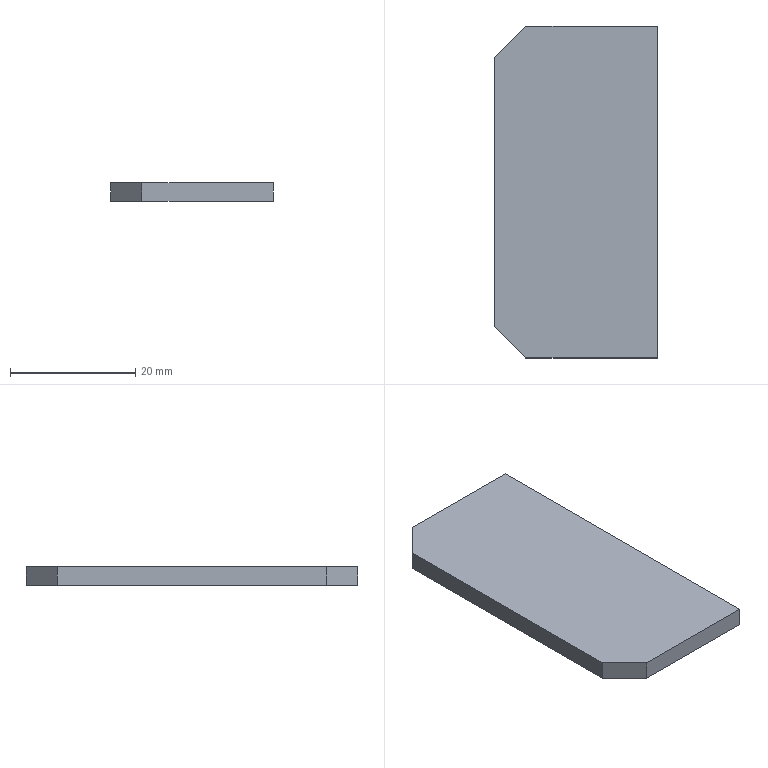Part | SolidWorks | features Chamfer 1, FlatPattern 1, SMBaseFlange 1, SheetMetal 1 | 1 solid | 8 faces | box 26 x 53 x 3 mm | volume 4059 mm3 | plane 8
STEP:
#1=CARTESIAN_POINT('',(26.,26.5,-3.));
#2=VERTEX_POINT('',#1);
#3=CARTESIAN_POINT('',(5.,26.5,-3.));
#4=VERTEX_POINT('',#3);
#5=CARTESIAN_POINT('',(26.,26.5,-3.));
#6=DIRECTION('',(-1.,0.,0.));
#7=VECTOR('',#6,1000.);
#8=LINE('',#5,#7);
#9=EDGE_CURVE('',#2,#4,#8,.T.);
#10=ORIENTED_EDGE('',*,*,#9,.T.);
#11=CARTESIAN_POINT('',(5.,26.5,0.));
#12=VERTEX_POINT('',#11);
#13=CARTESIAN_POINT('',(5.,26.5,-3.));
#14=DIRECTION('',(0.,0.,1.));
#15=VECTOR('',#14,1000.);
#16=LINE('',#13,#15);
#17=EDGE_CURVE('',#4,#12,#16,.T.);
#18=ORIENTED_EDGE('',*,*,#17,.T.);
#19=CARTESIAN_POINT('',(26.,26.5,0.));
#20=VERTEX_POINT('',#19);
#21=CARTESIAN_POINT('',(26.,26.5,0.));
#22=DIRECTION('',(-1.,0.,0.));
#23=VECTOR('',#22,1000.);
#24=LINE('',#21,#23);
#25=EDGE_CURVE('',#20,#12,#24,.T.);
#26=ORIENTED_EDGE('',*,*,#25,.F.);
#27=CARTESIAN_POINT('',(26.,26.5,-3.));
#28=DIRECTION('',(0.,0.,1.));
#29=VECTOR('',#28,1000.);
#30=LINE('',#27,#29);
#31=EDGE_CURVE('',#2,#20,#30,.T.);
#32=ORIENTED_EDGE('',*,*,#31,.F.);
#33=EDGE_LOOP('',(#10,#18,#26,#32));
#34=FACE_OUTER_BOUND('',#33,.T.);
#35=CARTESIAN_POINT('',(26.,26.5,-3.));
#36=DIRECTION('',(0.,1.,0.));
#37=DIRECTION('',(-1.,0.,0.));
#38=AXIS2_PLACEMENT_3D('',#35,#36,#37);
#39=PLANE('',#38);
#40=ADVANCED_FACE('',(#34),#39,.T.);
#41=CARTESIAN_POINT('',(26.,-26.5,0.));
#42=VERTEX_POINT('',#41);
#43=CARTESIAN_POINT('',(26.,-26.5,0.));
#44=DIRECTION('',(0.,1.,0.));
#45=VECTOR('',#44,1000.);
#46=LINE('',#43,#45);
#47=EDGE_CURVE('',#42,#20,#46,.T.);
#48=ORIENTED_EDGE('',*,*,#47,.F.);
#49=CARTESIAN_POINT('',(26.,-26.5,-3.));
#50=VERTEX_POINT('',#49);
#51=CARTESIAN_POINT('',(26.,-26.5,-3.));
#52=DIRECTION('',(0.,0.,1.));
#53=VECTOR('',#52,1000.);
#54=LINE('',#51,#53);
#55=EDGE_CURVE('',#50,#42,#54,.T.);
#56=ORIENTED_EDGE('',*,*,#55,.F.);
#57=CARTESIAN_POINT('',(26.,-26.5,-3.));
#58=DIRECTION('',(0.,1.,0.));
#59=VECTOR('',#58,1000.);
#60=LINE('',#57,#59);
#61=EDGE_CURVE('',#50,#2,#60,.T.);
#62=ORIENTED_EDGE('',*,*,#61,.T.);
#63=ORIENTED_EDGE('',*,*,#31,.T.);
#64=EDGE_LOOP('',(#48,#56,#62,#63));
#65=FACE_OUTER_BOUND('',#64,.T.);
#66=CARTESIAN_POINT('',(26.,-26.5,-3.));
#67=DIRECTION('',(1.,0.,0.));
#68=DIRECTION('',(0.,1.,0.));
#69=AXIS2_PLACEMENT_3D('',#66,#67,#68);
#70=PLANE('',#69);
#71=ADVANCED_FACE('',(#65),#70,.T.);
#72=CARTESIAN_POINT('',(5.,-26.5,0.));
#73=VERTEX_POINT('',#72);
#74=CARTESIAN_POINT('',(0.,-26.5,0.));
#75=DIRECTION('',(1.,0.,0.));
#76=VECTOR('',#75,1000.);
#77=LINE('',#74,#76);
#78=EDGE_CURVE('',#73,#42,#77,.T.);
#79=ORIENTED_EDGE('',*,*,#78,.F.);
#80=CARTESIAN_POINT('',(5.,-26.5,-3.));
#81=VERTEX_POINT('',#80);
#82=CARTESIAN_POINT('',(5.,-26.5,-3.));
#83=DIRECTION('',(0.,0.,-1.));
#84=VECTOR('',#83,1000.);
#85=LINE('',#82,#84);
#86=EDGE_CURVE('',#73,#81,#85,.T.);
#87=ORIENTED_EDGE('',*,*,#86,.T.);
#88=CARTESIAN_POINT('',(0.,-26.5,-3.));
#89=DIRECTION('',(1.,0.,0.));
#90=VECTOR('',#89,1000.);
#91=LINE('',#88,#90);
#92=EDGE_CURVE('',#81,#50,#91,.T.);
#93=ORIENTED_EDGE('',*,*,#92,.T.);
#94=ORIENTED_EDGE('',*,*,#55,.T.);
#95=EDGE_LOOP('',(#79,#87,#93,#94));
#96=FACE_OUTER_BOUND('',#95,.T.);
#97=CARTESIAN_POINT('',(0.,-26.5,-3.));
#98=DIRECTION('',(0.,-1.,0.));
#99=DIRECTION('',(0.,0.,-1.));
#100=AXIS2_PLACEMENT_3D('',#97,#98,#99);
#101=PLANE('',#100);
#102=ADVANCED_FACE('',(#96),#101,.T.);
#103=CARTESIAN_POINT('',(0.,21.5,-3.));
#104=VERTEX_POINT('',#103);
#105=CARTESIAN_POINT('',(0.,-21.5,-3.));
#106=VERTEX_POINT('',#105);
#107=CARTESIAN_POINT('',(0.,26.5,-3.));
#108=DIRECTION('',(0.,-1.,0.));
#109=VECTOR('',#108,1000.);
#110=LINE('',#107,#109);
#111=EDGE_CURVE('',#104,#106,#110,.T.);
#112=ORIENTED_EDGE('',*,*,#111,.T.);
#113=CARTESIAN_POINT('',(0.,-21.5,0.));
#114=VERTEX_POINT('',#113);
#115=CARTESIAN_POINT('',(0.,-21.5,-3.));
#116=DIRECTION('',(0.,0.,1.));
#117=VECTOR('',#116,1000.);
#118=LINE('',#115,#117);
#119=EDGE_CURVE('',#106,#114,#118,.T.);
#120=ORIENTED_EDGE('',*,*,#119,.T.);
#121=CARTESIAN_POINT('',(0.,21.5,0.));
#122=VERTEX_POINT('',#121);
#123=CARTESIAN_POINT('',(0.,26.5,0.));
#124=DIRECTION('',(0.,-1.,0.));
#125=VECTOR('',#124,1000.);
#126=LINE('',#123,#125);
#127=EDGE_CURVE('',#122,#114,#126,.T.);
#128=ORIENTED_EDGE('',*,*,#127,.F.);
#129=CARTESIAN_POINT('',(0.,21.5,-3.));
#130=DIRECTION('',(0.,0.,-1.));
#131=VECTOR('',#130,1000.);
#132=LINE('',#129,#131);
#133=EDGE_CURVE('',#122,#104,#132,.T.);
#134=ORIENTED_EDGE('',*,*,#133,.T.);
#135=EDGE_LOOP('',(#112,#120,#128,#134));
#136=FACE_OUTER_BOUND('',#135,.T.);
#137=CARTESIAN_POINT('',(0.,26.5,-3.));
#138=DIRECTION('',(-1.,0.,0.));
#139=DIRECTION('',(0.,-1.,0.));
#140=AXIS2_PLACEMENT_3D('',#137,#138,#139);
#141=PLANE('',#140);
#142=ADVANCED_FACE('',(#136),#141,.T.);
#143=ORIENTED_EDGE('',*,*,#92,.F.);
#144=CARTESIAN_POINT('',(0.,-21.5,-3.));
#145=DIRECTION('',(-0.7071,0.7071,0.));
#146=VECTOR('',#145,1000.);
#147=LINE('',#144,#146);
#148=EDGE_CURVE('',#81,#106,#147,.T.);
#149=ORIENTED_EDGE('',*,*,#148,.T.);
#150=ORIENTED_EDGE('',*,*,#111,.F.);
#151=CARTESIAN_POINT('',(5.,26.5,-3.));
#152=DIRECTION('',(0.7071,0.7071,0.));
#153=VECTOR('',#152,1000.);
#154=LINE('',#151,#153);
#155=EDGE_CURVE('',#104,#4,#154,.T.);
#156=ORIENTED_EDGE('',*,*,#155,.T.);
#157=ORIENTED_EDGE('',*,*,#9,.F.);
#158=ORIENTED_EDGE('',*,*,#61,.F.);
#159=EDGE_LOOP('',(#143,#149,#150,#156,#157,#158));
#160=FACE_OUTER_BOUND('',#159,.T.);
#161=CARTESIAN_POINT('',(0.,0.,-3.));
#162=DIRECTION('',(0.,0.,1.));
#163=DIRECTION('',(1.,0.,0.));
#164=AXIS2_PLACEMENT_3D('',#161,#162,#163);
#165=PLANE('',#164);
#166=ADVANCED_FACE('',(#160),#165,.F.);
#167=ORIENTED_EDGE('',*,*,#127,.T.);
#168=CARTESIAN_POINT('',(-10.75,-10.75,0.));
#169=DIRECTION('',(0.7071,-0.7071,0.));
#170=VECTOR('',#169,1000.);
#171=LINE('',#168,#170);
#172=EDGE_CURVE('',#114,#73,#171,.T.);
#173=ORIENTED_EDGE('',*,*,#172,.T.);
#174=ORIENTED_EDGE('',*,*,#78,.T.);
#175=ORIENTED_EDGE('',*,*,#47,.T.);
#176=ORIENTED_EDGE('',*,*,#25,.T.);
#177=CARTESIAN_POINT('',(-10.75,10.75,0.));
#178=DIRECTION('',(-0.7071,-0.7071,0.));
#179=VECTOR('',#178,1000.);
#180=LINE('',#177,#179);
#181=EDGE_CURVE('',#12,#122,#180,.T.);
#182=ORIENTED_EDGE('',*,*,#181,.T.);
#183=EDGE_LOOP('',(#167,#173,#174,#175,#176,#182));
#184=FACE_OUTER_BOUND('',#183,.T.);
#185=CARTESIAN_POINT('',(0.,0.,0.));
#186=DIRECTION('',(0.,0.,1.));
#187=DIRECTION('',(1.,0.,0.));
#188=AXIS2_PLACEMENT_3D('',#185,#186,#187);
#189=PLANE('',#188);
#190=ADVANCED_FACE('',(#184),#189,.T.);
#191=ORIENTED_EDGE('',*,*,#148,.F.);
#192=ORIENTED_EDGE('',*,*,#86,.F.);
#193=ORIENTED_EDGE('',*,*,#172,.F.);
#194=ORIENTED_EDGE('',*,*,#119,.F.);
#195=EDGE_LOOP('',(#191,#192,#193,#194));
#196=FACE_OUTER_BOUND('',#195,.T.);
#197=CARTESIAN_POINT('',(0.,-21.5,-3.));
#198=DIRECTION('',(0.7071,0.7071,0.));
#199=DIRECTION('',(0.,0.,1.));
#200=AXIS2_PLACEMENT_3D('',#197,#198,#199);
#201=PLANE('',#200);
#202=ADVANCED_FACE('',(#196),#201,.F.);
#203=ORIENTED_EDGE('',*,*,#155,.F.);
#204=ORIENTED_EDGE('',*,*,#133,.F.);
#205=ORIENTED_EDGE('',*,*,#181,.F.);
#206=ORIENTED_EDGE('',*,*,#17,.F.);
#207=EDGE_LOOP('',(#203,#204,#205,#206));
#208=FACE_OUTER_BOUND('',#207,.T.);
#209=CARTESIAN_POINT('',(5.,26.5,-3.));
#210=DIRECTION('',(0.7071,-0.7071,0.));
#211=DIRECTION('',(0.,0.,1.));
#212=AXIS2_PLACEMENT_3D('',#209,#210,#211);
#213=PLANE('',#212);
#214=ADVANCED_FACE('',(#208),#213,.F.);
#215=CLOSED_SHELL('',(#40,#71,#102,#142,#166,#190,#202,#214));
#216=MANIFOLD_SOLID_BREP('',#215);
#217=CARTESIAN_POINT('',(0.,0.,0.));
#218=DIRECTION('',(0.,0.,1.));
#219=DIRECTION('',(1.,0.,0.));
#220=AXIS2_PLACEMENT_3D('',#217,#218,#219);
#221=(LENGTH_UNIT()NAMED_UNIT(*)SI_UNIT(.MILLI.,.METRE.));
#222=UNCERTAINTY_MEASURE_WITH_UNIT(LENGTH_MEASURE(0.00001),#221,'','');
#223=(NAMED_UNIT(*)PLANE_ANGLE_UNIT()SI_UNIT($,.RADIAN.));
#224=(NAMED_UNIT(*)SI_UNIT($,.STERADIAN.)SOLID_ANGLE_UNIT());
#225=(GEOMETRIC_REPRESENTATION_CONTEXT(3)GLOBAL_UNCERTAINTY_ASSIGNED_CONTEXT((#222))GLOBAL_UNIT_ASSIGNED_CONTEXT((#221,#223,#224))REPRESENTATION_CONTEXT('',''));
#226=ADVANCED_BREP_SHAPE_REPRESENTATION('',(#216,#220),#225);